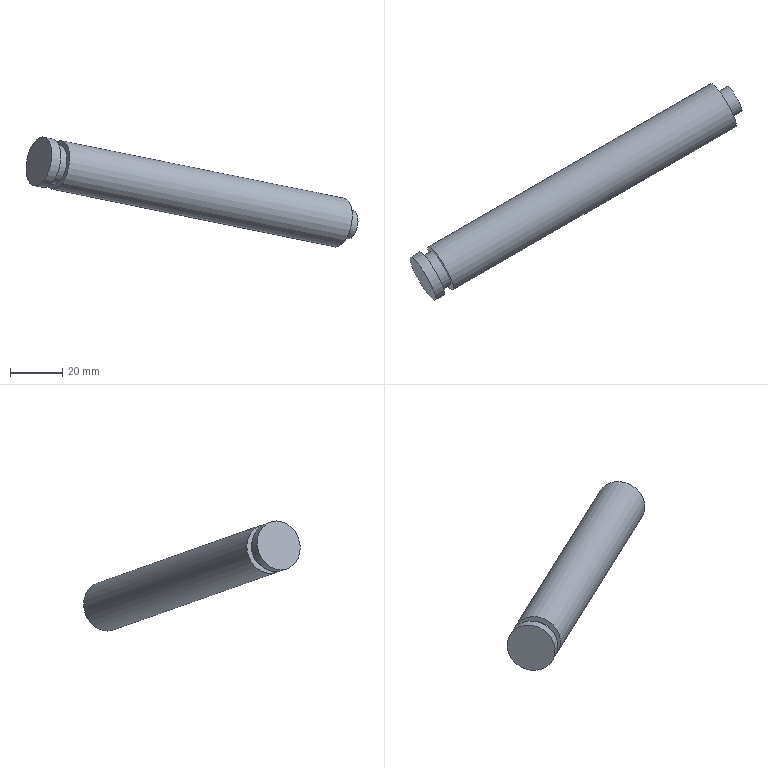Part | NX | features solid 2 | 1 solid | 9 faces | box 127.233 x 83.011 x 42.154 mm | volume 38324 mm3 | plane 5 | cylinder 4 | commonest cylinder face diameters 19 x2 11 x1 15 x1
STEP:
#1=CARTESIAN_POINT('',(-877.025,137.795,-54.328));
#2=VERTEX_POINT('',#1);
#3=CARTESIAN_POINT('',(-874.275,133.032,-54.328));
#4=DIRECTION('',(0.8529,0.4924,-0.1736));
#5=DIRECTION('',(-0.5,0.866,0.));
#6=AXIS2_PLACEMENT_3D('',#3,#4,#5);
#7=CIRCLE('',#6,5.5);
#8=EDGE_CURVE('',#2,#2,#7,.F.);
#9=ORIENTED_EDGE('',*,*,#8,.F.);
#10=EDGE_LOOP('',(#9));
#11=FACE_BOUND('',#10,.T.);
#12=CARTESIAN_POINT('',(-872.761,140.257,-55.197));
#13=VERTEX_POINT('',#12);
#14=CARTESIAN_POINT('',(-870.011,135.494,-55.197));
#15=DIRECTION('',(0.8529,0.4924,-0.1736));
#16=DIRECTION('',(-0.5,0.866,0.));
#17=AXIS2_PLACEMENT_3D('',#14,#15,#16);
#18=CIRCLE('',#17,5.5);
#19=EDGE_CURVE('',#13,#13,#18,.F.);
#20=ORIENTED_EDGE('',*,*,#19,.T.);
#21=EDGE_LOOP('',(#20));
#22=FACE_BOUND('',#21,.T.);
#23=CARTESIAN_POINT('',(-872.57,134.016,-54.676));
#24=DIRECTION('',(0.8529,0.4924,-0.1736));
#25=DIRECTION('',(0.2933,-0.727,-0.6209));
#26=AXIS2_PLACEMENT_3D('',#23,#24,#25);
#27=CYLINDRICAL_SURFACE('',#26,5.5);
#28=ADVANCED_FACE('',(#11,#22),#27,.T.);
#29=ORIENTED_EDGE('',*,*,#8,.T.);
#30=EDGE_LOOP('',(#29));
#31=FACE_BOUND('',#30,.T.);
#32=CARTESIAN_POINT('',(-879.025,141.259,-54.328));
#33=VERTEX_POINT('',#32);
#34=CARTESIAN_POINT('',(-874.275,133.032,-54.328));
#35=DIRECTION('',(0.8529,0.4924,-0.1736));
#36=DIRECTION('',(-0.5,0.866,0.));
#37=AXIS2_PLACEMENT_3D('',#34,#35,#36);
#38=CIRCLE('',#37,9.5);
#39=EDGE_CURVE('',#33,#33,#38,.T.);
#40=ORIENTED_EDGE('',*,*,#39,.T.);
#41=EDGE_LOOP('',(#40));
#42=FACE_BOUND('',#41,.T.);
#43=CARTESIAN_POINT('',(-874.275,133.032,-54.328));
#44=DIRECTION('',(0.8529,0.4924,-0.1736));
#45=DIRECTION('',(0.2933,-0.727,-0.6209));
#46=AXIS2_PLACEMENT_3D('',#43,#44,#45);
#47=PLANE('',#46);
#48=ADVANCED_FACE('',(#31,#42),#47,.T.);
#49=CARTESIAN_POINT('',(-983.982,69.609,-41.63));
#50=VERTEX_POINT('',#49);
#51=CARTESIAN_POINT('',(-982.59,70.496,-32.275));
#52=DIRECTION('',(0.8529,0.4924,-0.1736));
#53=DIRECTION('',(-0.1466,-0.09342,-0.9848));
#54=AXIS2_PLACEMENT_3D('',#51,#52,#53);
#55=CIRCLE('',#54,9.5);
#56=EDGE_CURVE('',#50,#50,#55,.T.);
#57=ORIENTED_EDGE('',*,*,#56,.T.);
#58=EDGE_LOOP('',(#57));
#59=FACE_BOUND('',#58,.T.);
#60=ORIENTED_EDGE('',*,*,#39,.F.);
#61=EDGE_LOOP('',(#60));
#62=FACE_BOUND('',#61,.T.);
#63=CARTESIAN_POINT('',(-957.857,84.776,-37.311));
#64=DIRECTION('',(0.8529,0.4924,-0.1736));
#65=DIRECTION('',(0.2933,-0.727,-0.6209));
#66=AXIS2_PLACEMENT_3D('',#63,#64,#65);
#67=CYLINDRICAL_SURFACE('',#66,9.5);
#68=ADVANCED_FACE('',(#59,#62),#67,.T.);
#69=CARTESIAN_POINT('',(-983.689,69.796,-39.661));
#70=VERTEX_POINT('',#69);
#71=CARTESIAN_POINT('',(-982.59,70.496,-32.275));
#72=DIRECTION('',(0.8529,0.4924,-0.1736));
#73=DIRECTION('',(-0.1466,-0.09342,-0.9848));
#74=AXIS2_PLACEMENT_3D('',#71,#72,#73);
#75=CIRCLE('',#74,7.5);
#76=EDGE_CURVE('',#70,#70,#75,.T.);
#77=ORIENTED_EDGE('',*,*,#76,.T.);
#78=EDGE_LOOP('',(#77));
#79=FACE_BOUND('',#78,.T.);
#80=ORIENTED_EDGE('',*,*,#56,.F.);
#81=EDGE_LOOP('',(#80));
#82=FACE_BOUND('',#81,.T.);
#83=CARTESIAN_POINT('',(-982.59,70.496,-32.275));
#84=DIRECTION('',(0.8529,0.4924,-0.1736));
#85=DIRECTION('',(0.2933,-0.727,-0.6209));
#86=AXIS2_PLACEMENT_3D('',#83,#84,#85);
#87=PLANE('',#86);
#88=ADVANCED_FACE('',(#79,#82),#87,.F.);
#89=CARTESIAN_POINT('',(-987.101,67.826,-38.966));
#90=VERTEX_POINT('',#89);
#91=CARTESIAN_POINT('',(-986.001,68.527,-31.58));
#92=DIRECTION('',(0.8529,0.4924,-0.1736));
#93=DIRECTION('',(-0.1466,-0.09342,-0.9848));
#94=AXIS2_PLACEMENT_3D('',#91,#92,#93);
#95=CIRCLE('',#94,7.5);
#96=EDGE_CURVE('',#90,#90,#95,.T.);
#97=ORIENTED_EDGE('',*,*,#96,.T.);
#98=EDGE_LOOP('',(#97));
#99=FACE_BOUND('',#98,.T.);
#100=ORIENTED_EDGE('',*,*,#76,.F.);
#101=EDGE_LOOP('',(#100));
#102=FACE_BOUND('',#101,.T.);
#103=CARTESIAN_POINT('',(-957.857,84.776,-37.311));
#104=DIRECTION('',(0.8529,0.4924,-0.1736));
#105=DIRECTION('',(0.2933,-0.727,-0.6209));
#106=AXIS2_PLACEMENT_3D('',#103,#104,#105);
#107=CYLINDRICAL_SURFACE('',#106,7.5);
#108=ADVANCED_FACE('',(#99,#102),#107,.T.);
#109=ORIENTED_EDGE('',*,*,#96,.F.);
#110=EDGE_LOOP('',(#109));
#111=FACE_BOUND('',#110,.T.);
#112=CARTESIAN_POINT('',(-987.394,67.639,-40.936));
#113=VERTEX_POINT('',#112);
#114=CARTESIAN_POINT('',(-986.001,68.527,-31.58));
#115=DIRECTION('',(0.8529,0.4924,-0.1736));
#116=DIRECTION('',(-0.1466,-0.09342,-0.9848));
#117=AXIS2_PLACEMENT_3D('',#114,#115,#116);
#118=CIRCLE('',#117,9.5);
#119=EDGE_CURVE('',#113,#113,#118,.T.);
#120=ORIENTED_EDGE('',*,*,#119,.T.);
#121=EDGE_LOOP('',(#120));
#122=FACE_BOUND('',#121,.T.);
#123=CARTESIAN_POINT('',(-986.001,68.527,-31.58));
#124=DIRECTION('',(0.8529,0.4924,-0.1736));
#125=DIRECTION('',(0.2933,-0.727,-0.6209));
#126=AXIS2_PLACEMENT_3D('',#123,#124,#125);
#127=PLANE('',#126);
#128=ADVANCED_FACE('',(#111,#122),#127,.T.);
#129=CARTESIAN_POINT('',(-988.02,67.445,-21.53));
#130=VERTEX_POINT('',#129);
#131=CARTESIAN_POINT('',(-989.413,66.557,-30.886));
#132=DIRECTION('',(-0.8529,-0.4924,0.1736));
#133=DIRECTION('',(0.1466,0.09342,0.9848));
#134=AXIS2_PLACEMENT_3D('',#131,#132,#133);
#135=CIRCLE('',#134,9.5);
#136=EDGE_CURVE('',#130,#130,#135,.T.);
#137=ORIENTED_EDGE('',*,*,#136,.T.);
#138=EDGE_LOOP('',(#137));
#139=FACE_BOUND('',#138,.T.);
#140=CARTESIAN_POINT('',(-989.413,66.557,-30.886));
#141=DIRECTION('',(-0.8529,-0.4924,0.1736));
#142=DIRECTION('',(-0.2933,0.727,0.6209));
#143=AXIS2_PLACEMENT_3D('',#140,#141,#142);
#144=PLANE('',#143);
#145=ADVANCED_FACE('',(#139),#144,.T.);
#146=ORIENTED_EDGE('',*,*,#136,.F.);
#147=EDGE_LOOP('',(#146));
#148=FACE_BOUND('',#147,.T.);
#149=ORIENTED_EDGE('',*,*,#119,.F.);
#150=EDGE_LOOP('',(#149));
#151=FACE_BOUND('',#150,.T.);
#152=CARTESIAN_POINT('',(-957.857,84.776,-37.311));
#153=DIRECTION('',(0.8529,0.4924,-0.1736));
#154=DIRECTION('',(0.2933,-0.727,-0.6209));
#155=AXIS2_PLACEMENT_3D('',#152,#153,#154);
#156=CYLINDRICAL_SURFACE('',#155,9.5);
#157=ADVANCED_FACE('',(#148,#151),#156,.T.);
#158=ORIENTED_EDGE('',*,*,#19,.F.);
#159=EDGE_LOOP('',(#158));
#160=FACE_BOUND('',#159,.T.);
#161=CARTESIAN_POINT('',(-868.499,133.819,-52.521));
#162=DIRECTION('',(0.8529,0.4924,-0.1736));
#163=DIRECTION('',(-0.432,0.4786,-0.7644));
#164=AXIS2_PLACEMENT_3D('',#161,#162,#163);
#165=PLANE('',#164);
#166=ADVANCED_FACE('',(#160),#165,.T.);
#167=CLOSED_SHELL('',(#28,#48,#68,#88,#108,#128,#145,#157,#166));
#168=MANIFOLD_SOLID_BREP('',#167);
#169=(LENGTH_UNIT()NAMED_UNIT(*)SI_UNIT(.MILLI.,.METRE.));
#170=UNCERTAINTY_MEASURE_WITH_UNIT(LENGTH_MEASURE(0.00001),#169,'','');
#171=(NAMED_UNIT(*)PLANE_ANGLE_UNIT()SI_UNIT($,.RADIAN.));
#172=(NAMED_UNIT(*)SI_UNIT($,.STERADIAN.)SOLID_ANGLE_UNIT());
#173=(GEOMETRIC_REPRESENTATION_CONTEXT(3)GLOBAL_UNCERTAINTY_ASSIGNED_CONTEXT((#170))GLOBAL_UNIT_ASSIGNED_CONTEXT((#169,#171,#172))REPRESENTATION_CONTEXT('',''));
#174=ADVANCED_BREP_SHAPE_REPRESENTATION('',(#168),#173);